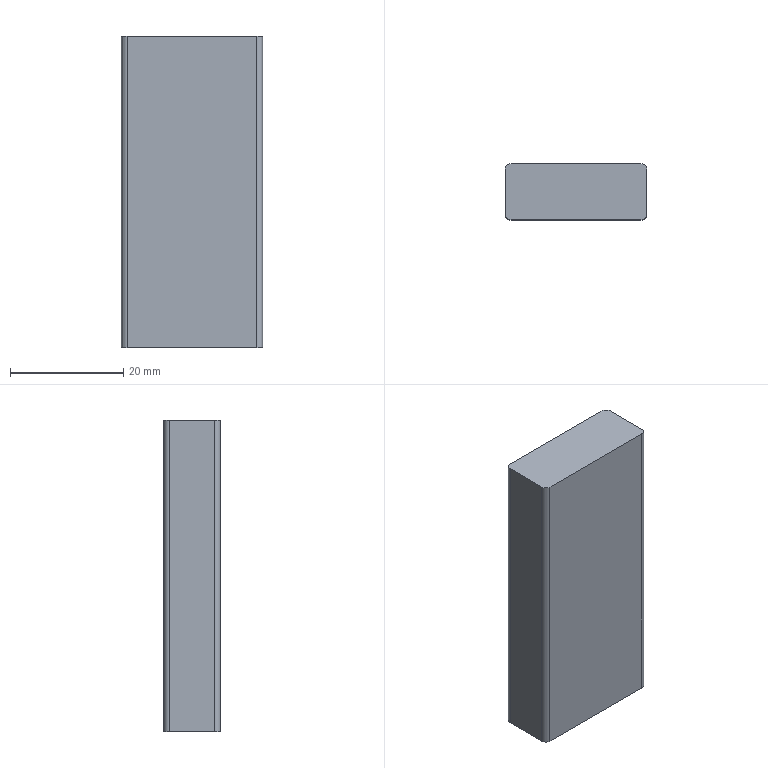Part | STEP file | 1 solid | 10 faces | box 24.97 x 9.97 x 55 mm | volume 13645 mm3 | plane 6 | cylinder 4 | commonest cylinder face diameters 2 x4
STEP:
#1=CARTESIAN_POINT('',(0.,0.,0.));
#2=DIRECTION('',(0.,0.,1.));
#3=DIRECTION('',(1.,0.,0.));
#4=AXIS2_PLACEMENT_3D('',#1,#2,#3);
#5=CARTESIAN_POINT('',(1277.232,396.43,43.619));
#6=VERTEX_POINT('',#5);
#7=CARTESIAN_POINT('',(1277.232,388.46,43.619));
#8=VERTEX_POINT('',#7);
#9=CARTESIAN_POINT('',(1277.232,397.445,43.619));
#10=DIRECTION('',(0.,-1.,0.));
#11=VECTOR('',#10,1.);
#12=LINE('',#9,#11);
#13=CARTESIAN_POINT('',(20683.4,-3580.314,43.619));
#14=DIRECTION('',(0.,0.,1.));
#15=DIRECTION('',(1.,0.,0.));
#16=AXIS2_PLACEMENT_3D('',#13,#14,#15);
#17=PLANE('',#16);
#18=CARTESIAN_POINT('',(-19406.168,3977.759));
#19=DIRECTION('',(0.,-1.));
#20=VECTOR('',#19,1.);
#21=LINE('',#18,#20);
#22=(GEOMETRIC_REPRESENTATION_CONTEXT(2)PARAMETRIC_REPRESENTATION_CONTEXT()REPRESENTATION_CONTEXT('',''));
#23=DEFINITIONAL_REPRESENTATION('',(#21),#22);
#24=PCURVE('',#17,#23);
#25=CARTESIAN_POINT('',(1277.232,397.445,426.319));
#26=DIRECTION('',(1.,0.,0.));
#27=DIRECTION('',(0.,0.,-1.));
#28=AXIS2_PLACEMENT_3D('',#25,#26,#27);
#29=PLANE('',#28);
#30=CARTESIAN_POINT('',(382.7,0.));
#31=DIRECTION('',(0.,-1.));
#32=VECTOR('',#31,1.);
#33=LINE('',#30,#32);
#34=(GEOMETRIC_REPRESENTATION_CONTEXT(2)PARAMETRIC_REPRESENTATION_CONTEXT()REPRESENTATION_CONTEXT('',''));
#35=DEFINITIONAL_REPRESENTATION('',(#33),#34);
#36=PCURVE('',#29,#35);
#37=SURFACE_CURVE('',#12,(#24,#36),.PCURVE_S1.);
#38=EDGE_CURVE('',#6,#8,#37,.T.);
#39=ORIENTED_EDGE('',*,*,#38,.F.);
#40=CARTESIAN_POINT('',(1276.232,397.43,43.619));
#41=VERTEX_POINT('',#40);
#42=CARTESIAN_POINT('',(1276.232,396.43,43.619));
#43=DIRECTION('',(0.,0.,1.));
#44=DIRECTION('',(-1.,0.,0.));
#45=AXIS2_PLACEMENT_3D('',#42,#43,#44);
#46=CIRCLE('',#45,1.);
#47=CARTESIAN_POINT('',(-19407.168,3976.744));
#48=DIRECTION('',(-1.,0.));
#49=AXIS2_PLACEMENT_2D('',#47,#48);
#50=CIRCLE('',#49,1.);
#51=(GEOMETRIC_REPRESENTATION_CONTEXT(2)PARAMETRIC_REPRESENTATION_CONTEXT()REPRESENTATION_CONTEXT('',''));
#52=DEFINITIONAL_REPRESENTATION('',(#50),#51);
#53=PCURVE('',#17,#52);
#54=CARTESIAN_POINT('',(1276.232,396.43,426.319));
#55=DIRECTION('',(0.,0.,-1.));
#56=DIRECTION('',(-1.,0.,0.));
#57=AXIS2_PLACEMENT_3D('',#54,#55,#56);
#58=CYLINDRICAL_SURFACE('',#57,1.);
#59=CARTESIAN_POINT('',(6.283,382.7));
#60=DIRECTION('',(-1.,0.));
#61=VECTOR('',#60,1.);
#62=LINE('',#59,#61);
#63=(GEOMETRIC_REPRESENTATION_CONTEXT(2)PARAMETRIC_REPRESENTATION_CONTEXT()REPRESENTATION_CONTEXT('',''));
#64=DEFINITIONAL_REPRESENTATION('',(#62),#63);
#65=PCURVE('',#58,#64);
#66=SURFACE_CURVE('',#46,(#53,#65),.PCURVE_S1.);
#67=EDGE_CURVE('',#6,#41,#66,.T.);
#68=ORIENTED_EDGE('',*,*,#67,.T.);
#69=CARTESIAN_POINT('',(1253.262,397.43,43.619));
#70=VERTEX_POINT('',#69);
#71=CARTESIAN_POINT('',(1252.247,397.43,43.619));
#72=DIRECTION('',(1.,0.,0.));
#73=VECTOR('',#72,1.);
#74=LINE('',#71,#73);
#75=CARTESIAN_POINT('',(-19431.153,3977.744));
#76=DIRECTION('',(1.,0.));
#77=VECTOR('',#76,1.);
#78=LINE('',#75,#77);
#79=(GEOMETRIC_REPRESENTATION_CONTEXT(2)PARAMETRIC_REPRESENTATION_CONTEXT()REPRESENTATION_CONTEXT('',''));
#80=DEFINITIONAL_REPRESENTATION('',(#78),#79);
#81=PCURVE('',#17,#80);
#82=CARTESIAN_POINT('',(1252.247,397.43,426.319));
#83=DIRECTION('',(0.,1.,0.));
#84=DIRECTION('',(0.,0.,-1.));
#85=AXIS2_PLACEMENT_3D('',#82,#83,#84);
#86=PLANE('',#85);
#87=CARTESIAN_POINT('',(382.7,0.));
#88=DIRECTION('',(0.,-1.));
#89=VECTOR('',#88,1.);
#90=LINE('',#87,#89);
#91=(GEOMETRIC_REPRESENTATION_CONTEXT(2)PARAMETRIC_REPRESENTATION_CONTEXT()REPRESENTATION_CONTEXT('',''));
#92=DEFINITIONAL_REPRESENTATION('',(#90),#91);
#93=PCURVE('',#86,#92);
#94=SURFACE_CURVE('',#74,(#81,#93),.PCURVE_S1.);
#95=EDGE_CURVE('',#70,#41,#94,.T.);
#96=ORIENTED_EDGE('',*,*,#95,.F.);
#97=CARTESIAN_POINT('',(1252.262,396.43,43.619));
#98=VERTEX_POINT('',#97);
#99=CARTESIAN_POINT('',(1253.262,396.43,43.619));
#100=DIRECTION('',(0.,0.,1.));
#101=DIRECTION('',(-1.,0.,0.));
#102=AXIS2_PLACEMENT_3D('',#99,#100,#101);
#103=CIRCLE('',#102,1.);
#104=CARTESIAN_POINT('',(-19430.138,3976.744));
#105=DIRECTION('',(-1.,0.));
#106=AXIS2_PLACEMENT_2D('',#104,#105);
#107=CIRCLE('',#106,1.);
#108=(GEOMETRIC_REPRESENTATION_CONTEXT(2)PARAMETRIC_REPRESENTATION_CONTEXT()REPRESENTATION_CONTEXT('',''));
#109=DEFINITIONAL_REPRESENTATION('',(#107),#108);
#110=PCURVE('',#17,#109);
#111=CARTESIAN_POINT('',(1253.262,396.43,426.319));
#112=DIRECTION('',(0.,0.,-1.));
#113=DIRECTION('',(-1.,0.,0.));
#114=AXIS2_PLACEMENT_3D('',#111,#112,#113);
#115=CYLINDRICAL_SURFACE('',#114,1.);
#116=CARTESIAN_POINT('',(6.283,382.7));
#117=DIRECTION('',(-1.,0.));
#118=VECTOR('',#117,1.);
#119=LINE('',#116,#118);
#120=(GEOMETRIC_REPRESENTATION_CONTEXT(2)PARAMETRIC_REPRESENTATION_CONTEXT()REPRESENTATION_CONTEXT('',''));
#121=DEFINITIONAL_REPRESENTATION('',(#119),#120);
#122=PCURVE('',#115,#121);
#123=SURFACE_CURVE('',#103,(#110,#122),.PCURVE_S1.);
#124=EDGE_CURVE('',#70,#98,#123,.T.);
#125=ORIENTED_EDGE('',*,*,#124,.T.);
#126=CARTESIAN_POINT('',(1252.262,388.46,43.619));
#127=VERTEX_POINT('',#126);
#128=CARTESIAN_POINT('',(1252.262,387.445,43.619));
#129=DIRECTION('',(0.,1.,0.));
#130=VECTOR('',#129,1.);
#131=LINE('',#128,#130);
#132=CARTESIAN_POINT('',(-19431.138,3967.759));
#133=DIRECTION('',(0.,1.));
#134=VECTOR('',#133,1.);
#135=LINE('',#132,#134);
#136=(GEOMETRIC_REPRESENTATION_CONTEXT(2)PARAMETRIC_REPRESENTATION_CONTEXT()REPRESENTATION_CONTEXT('',''));
#137=DEFINITIONAL_REPRESENTATION('',(#135),#136);
#138=PCURVE('',#17,#137);
#139=CARTESIAN_POINT('',(1252.262,387.445,426.319));
#140=DIRECTION('',(-1.,0.,0.));
#141=DIRECTION('',(0.,0.,1.));
#142=AXIS2_PLACEMENT_3D('',#139,#140,#141);
#143=PLANE('',#142);
#144=CARTESIAN_POINT('',(-382.7,0.));
#145=DIRECTION('',(0.,1.));
#146=VECTOR('',#145,1.);
#147=LINE('',#144,#146);
#148=(GEOMETRIC_REPRESENTATION_CONTEXT(2)PARAMETRIC_REPRESENTATION_CONTEXT()REPRESENTATION_CONTEXT('',''));
#149=DEFINITIONAL_REPRESENTATION('',(#147),#148);
#150=PCURVE('',#143,#149);
#151=SURFACE_CURVE('',#131,(#138,#150),.PCURVE_S1.);
#152=EDGE_CURVE('',#127,#98,#151,.T.);
#153=ORIENTED_EDGE('',*,*,#152,.F.);
#154=CARTESIAN_POINT('',(1253.262,387.46,43.619));
#155=VERTEX_POINT('',#154);
#156=CARTESIAN_POINT('',(1253.262,388.46,43.619));
#157=DIRECTION('',(0.,0.,1.));
#158=DIRECTION('',(-1.,0.,0.));
#159=AXIS2_PLACEMENT_3D('',#156,#157,#158);
#160=CIRCLE('',#159,1.);
#161=CARTESIAN_POINT('',(-19430.138,3968.774));
#162=DIRECTION('',(-1.,0.));
#163=AXIS2_PLACEMENT_2D('',#161,#162);
#164=CIRCLE('',#163,1.);
#165=(GEOMETRIC_REPRESENTATION_CONTEXT(2)PARAMETRIC_REPRESENTATION_CONTEXT()REPRESENTATION_CONTEXT('',''));
#166=DEFINITIONAL_REPRESENTATION('',(#164),#165);
#167=PCURVE('',#17,#166);
#168=CARTESIAN_POINT('',(1253.262,388.46,426.319));
#169=DIRECTION('',(0.,0.,-1.));
#170=DIRECTION('',(-1.,0.,0.));
#171=AXIS2_PLACEMENT_3D('',#168,#169,#170);
#172=CYLINDRICAL_SURFACE('',#171,1.);
#173=CARTESIAN_POINT('',(6.283,382.7));
#174=DIRECTION('',(-1.,0.));
#175=VECTOR('',#174,1.);
#176=LINE('',#173,#175);
#177=(GEOMETRIC_REPRESENTATION_CONTEXT(2)PARAMETRIC_REPRESENTATION_CONTEXT()REPRESENTATION_CONTEXT('',''));
#178=DEFINITIONAL_REPRESENTATION('',(#176),#177);
#179=PCURVE('',#172,#178);
#180=SURFACE_CURVE('',#160,(#167,#179),.PCURVE_S1.);
#181=EDGE_CURVE('',#127,#155,#180,.T.);
#182=ORIENTED_EDGE('',*,*,#181,.T.);
#183=CARTESIAN_POINT('',(1276.232,387.46,43.619));
#184=VERTEX_POINT('',#183);
#185=CARTESIAN_POINT('',(1277.247,387.46,43.619));
#186=DIRECTION('',(-1.,0.,0.));
#187=VECTOR('',#186,1.);
#188=LINE('',#185,#187);
#189=CARTESIAN_POINT('',(-19406.153,3967.774));
#190=DIRECTION('',(-1.,0.));
#191=VECTOR('',#190,1.);
#192=LINE('',#189,#191);
#193=(GEOMETRIC_REPRESENTATION_CONTEXT(2)PARAMETRIC_REPRESENTATION_CONTEXT()REPRESENTATION_CONTEXT('',''));
#194=DEFINITIONAL_REPRESENTATION('',(#192),#193);
#195=PCURVE('',#17,#194);
#196=CARTESIAN_POINT('',(1277.247,387.46,426.319));
#197=DIRECTION('',(0.,-1.,0.));
#198=DIRECTION('',(0.,0.,1.));
#199=AXIS2_PLACEMENT_3D('',#196,#197,#198);
#200=PLANE('',#199);
#201=CARTESIAN_POINT('',(-382.7,0.));
#202=DIRECTION('',(0.,1.));
#203=VECTOR('',#202,1.);
#204=LINE('',#201,#203);
#205=(GEOMETRIC_REPRESENTATION_CONTEXT(2)PARAMETRIC_REPRESENTATION_CONTEXT()REPRESENTATION_CONTEXT('',''));
#206=DEFINITIONAL_REPRESENTATION('',(#204),#205);
#207=PCURVE('',#200,#206);
#208=SURFACE_CURVE('',#188,(#195,#207),.PCURVE_S1.);
#209=EDGE_CURVE('',#184,#155,#208,.T.);
#210=ORIENTED_EDGE('',*,*,#209,.F.);
#211=CARTESIAN_POINT('',(1276.232,388.46,43.619));
#212=DIRECTION('',(0.,0.,1.));
#213=DIRECTION('',(-1.,0.,0.));
#214=AXIS2_PLACEMENT_3D('',#211,#212,#213);
#215=CIRCLE('',#214,1.);
#216=CARTESIAN_POINT('',(-19407.168,3968.774));
#217=DIRECTION('',(-1.,0.));
#218=AXIS2_PLACEMENT_2D('',#216,#217);
#219=CIRCLE('',#218,1.);
#220=(GEOMETRIC_REPRESENTATION_CONTEXT(2)PARAMETRIC_REPRESENTATION_CONTEXT()REPRESENTATION_CONTEXT('',''));
#221=DEFINITIONAL_REPRESENTATION('',(#219),#220);
#222=PCURVE('',#17,#221);
#223=CARTESIAN_POINT('',(1276.232,388.46,426.319));
#224=DIRECTION('',(0.,0.,-1.));
#225=DIRECTION('',(-1.,0.,0.));
#226=AXIS2_PLACEMENT_3D('',#223,#224,#225);
#227=CYLINDRICAL_SURFACE('',#226,1.);
#228=CARTESIAN_POINT('',(6.283,382.7));
#229=DIRECTION('',(-1.,0.));
#230=VECTOR('',#229,1.);
#231=LINE('',#228,#230);
#232=(GEOMETRIC_REPRESENTATION_CONTEXT(2)PARAMETRIC_REPRESENTATION_CONTEXT()REPRESENTATION_CONTEXT('',''));
#233=DEFINITIONAL_REPRESENTATION('',(#231),#232);
#234=PCURVE('',#227,#233);
#235=SURFACE_CURVE('',#215,(#222,#234),.PCURVE_S1.);
#236=EDGE_CURVE('',#184,#8,#235,.T.);
#237=ORIENTED_EDGE('',*,*,#236,.T.);
#238=EDGE_LOOP('',(#39,#68,#96,#125,#153,#182,#210,#237));
#239=FACE_BOUND('',#238,.T.);
#240=ADVANCED_FACE('',(#239),#17,.T.);
#241=ORIENTED_EDGE('',*,*,#152,.T.);
#242=CARTESIAN_POINT('',(1252.262,396.43,-11.381));
#243=VERTEX_POINT('',#242);
#244=CARTESIAN_POINT('',(1252.262,396.43,426.319));
#245=DIRECTION('',(0.,0.,-1.));
#246=VECTOR('',#245,1.);
#247=LINE('',#244,#246);
#248=CARTESIAN_POINT('',(0.,8.985));
#249=DIRECTION('',(-1.,0.));
#250=VECTOR('',#249,1.);
#251=LINE('',#248,#250);
#252=(GEOMETRIC_REPRESENTATION_CONTEXT(2)PARAMETRIC_REPRESENTATION_CONTEXT()REPRESENTATION_CONTEXT('',''));
#253=DEFINITIONAL_REPRESENTATION('',(#251),#252);
#254=PCURVE('',#143,#253);
#255=CARTESIAN_POINT('',(0.,0.));
#256=DIRECTION('',(0.,1.));
#257=VECTOR('',#256,1.);
#258=LINE('',#255,#257);
#259=(GEOMETRIC_REPRESENTATION_CONTEXT(2)PARAMETRIC_REPRESENTATION_CONTEXT()REPRESENTATION_CONTEXT('',''));
#260=DEFINITIONAL_REPRESENTATION('',(#258),#259);
#261=PCURVE('',#115,#260);
#262=SURFACE_CURVE('',#247,(#254,#261),.PCURVE_S1.);
#263=EDGE_CURVE('',#98,#243,#262,.T.);
#264=ORIENTED_EDGE('',*,*,#263,.T.);
#265=CARTESIAN_POINT('',(1252.262,388.46,-11.381));
#266=VERTEX_POINT('',#265);
#267=CARTESIAN_POINT('',(1252.262,-3580.314,-11.381));
#268=DIRECTION('',(0.,1.,0.));
#269=VECTOR('',#268,1.);
#270=LINE('',#267,#269);
#271=CARTESIAN_POINT('',(-437.7,-3967.759));
#272=DIRECTION('',(0.,1.));
#273=VECTOR('',#272,1.);
#274=LINE('',#271,#273);
#275=(GEOMETRIC_REPRESENTATION_CONTEXT(2)PARAMETRIC_REPRESENTATION_CONTEXT()REPRESENTATION_CONTEXT('',''));
#276=DEFINITIONAL_REPRESENTATION('',(#274),#275);
#277=PCURVE('',#143,#276);
#278=CARTESIAN_POINT('',(18446.131,-3580.314,-11.381));
#279=DIRECTION('',(0.,0.,-1.));
#280=DIRECTION('',(-1.,0.,0.));
#281=AXIS2_PLACEMENT_3D('',#278,#279,#280);
#282=PLANE('',#281);
#283=CARTESIAN_POINT('',(17193.869,0.));
#284=DIRECTION('',(0.,1.));
#285=VECTOR('',#284,1.);
#286=LINE('',#283,#285);
#287=(GEOMETRIC_REPRESENTATION_CONTEXT(2)PARAMETRIC_REPRESENTATION_CONTEXT()REPRESENTATION_CONTEXT('',''));
#288=DEFINITIONAL_REPRESENTATION('',(#286),#287);
#289=PCURVE('',#282,#288);
#290=SURFACE_CURVE('',#270,(#277,#289),.PCURVE_S1.);
#291=EDGE_CURVE('',#266,#243,#290,.T.);
#292=ORIENTED_EDGE('',*,*,#291,.F.);
#293=CARTESIAN_POINT('',(1252.262,388.46,426.319));
#294=DIRECTION('',(0.,0.,1.));
#295=VECTOR('',#294,1.);
#296=LINE('',#293,#295);
#297=CARTESIAN_POINT('',(0.,1.015));
#298=DIRECTION('',(1.,0.));
#299=VECTOR('',#298,1.);
#300=LINE('',#297,#299);
#301=(GEOMETRIC_REPRESENTATION_CONTEXT(2)PARAMETRIC_REPRESENTATION_CONTEXT()REPRESENTATION_CONTEXT('',''));
#302=DEFINITIONAL_REPRESENTATION('',(#300),#301);
#303=PCURVE('',#143,#302);
#304=CARTESIAN_POINT('',(6.283,0.));
#305=DIRECTION('',(0.,-1.));
#306=VECTOR('',#305,1.);
#307=LINE('',#304,#306);
#308=(GEOMETRIC_REPRESENTATION_CONTEXT(2)PARAMETRIC_REPRESENTATION_CONTEXT()REPRESENTATION_CONTEXT('',''));
#309=DEFINITIONAL_REPRESENTATION('',(#307),#308);
#310=PCURVE('',#172,#309);
#311=SURFACE_CURVE('',#296,(#303,#310),.PCURVE_S1.);
#312=EDGE_CURVE('',#266,#127,#311,.T.);
#313=ORIENTED_EDGE('',*,*,#312,.T.);
#314=EDGE_LOOP('',(#241,#264,#292,#313));
#315=FACE_BOUND('',#314,.T.);
#316=ADVANCED_FACE('',(#315),#143,.T.);
#317=CARTESIAN_POINT('',(1253.262,397.43,-11.381));
#318=VERTEX_POINT('',#317);
#319=CARTESIAN_POINT('',(1276.232,397.43,-11.381));
#320=VERTEX_POINT('',#319);
#321=CARTESIAN_POINT('',(18446.131,397.43,-11.381));
#322=DIRECTION('',(1.,0.,0.));
#323=VECTOR('',#322,1.);
#324=LINE('',#321,#323);
#325=CARTESIAN_POINT('',(0.,3977.744));
#326=DIRECTION('',(-1.,0.));
#327=VECTOR('',#326,1.);
#328=LINE('',#325,#327);
#329=(GEOMETRIC_REPRESENTATION_CONTEXT(2)PARAMETRIC_REPRESENTATION_CONTEXT()REPRESENTATION_CONTEXT('',''));
#330=DEFINITIONAL_REPRESENTATION('',(#328),#329);
#331=PCURVE('',#282,#330);
#332=CARTESIAN_POINT('',(437.7,-17193.884));
#333=DIRECTION('',(0.,-1.));
#334=VECTOR('',#333,1.);
#335=LINE('',#332,#334);
#336=(GEOMETRIC_REPRESENTATION_CONTEXT(2)PARAMETRIC_REPRESENTATION_CONTEXT()REPRESENTATION_CONTEXT('',''));
#337=DEFINITIONAL_REPRESENTATION('',(#335),#336);
#338=PCURVE('',#86,#337);
#339=SURFACE_CURVE('',#324,(#331,#338),.PCURVE_S1.);
#340=EDGE_CURVE('',#318,#320,#339,.T.);
#341=ORIENTED_EDGE('',*,*,#340,.T.);
#342=CARTESIAN_POINT('',(1277.232,396.43,-11.381));
#343=VERTEX_POINT('',#342);
#344=CARTESIAN_POINT('',(1276.232,396.43,-11.381));
#345=DIRECTION('',(0.,0.,-1.));
#346=DIRECTION('',(-1.,0.,0.));
#347=AXIS2_PLACEMENT_3D('',#344,#345,#346);
#348=CIRCLE('',#347,1.);
#349=CARTESIAN_POINT('',(17169.899,3976.744));
#350=DIRECTION('',(1.,0.));
#351=AXIS2_PLACEMENT_2D('',#349,#350);
#352=CIRCLE('',#351,1.);
#353=(GEOMETRIC_REPRESENTATION_CONTEXT(2)PARAMETRIC_REPRESENTATION_CONTEXT()REPRESENTATION_CONTEXT('',''));
#354=DEFINITIONAL_REPRESENTATION('',(#352),#353);
#355=PCURVE('',#282,#354);
#356=CARTESIAN_POINT('',(0.,437.7));
#357=DIRECTION('',(1.,0.));
#358=VECTOR('',#357,1.);
#359=LINE('',#356,#358);
#360=(GEOMETRIC_REPRESENTATION_CONTEXT(2)PARAMETRIC_REPRESENTATION_CONTEXT()REPRESENTATION_CONTEXT('',''));
#361=DEFINITIONAL_REPRESENTATION('',(#359),#360);
#362=PCURVE('',#58,#361);
#363=SURFACE_CURVE('',#348,(#355,#362),.PCURVE_S1.);
#364=EDGE_CURVE('',#320,#343,#363,.T.);
#365=ORIENTED_EDGE('',*,*,#364,.T.);
#366=CARTESIAN_POINT('',(1277.232,388.46,-11.381));
#367=VERTEX_POINT('',#366);
#368=CARTESIAN_POINT('',(1277.232,-3580.314,-11.381));
#369=DIRECTION('',(0.,-1.,0.));
#370=VECTOR('',#369,1.);
#371=LINE('',#368,#370);
#372=CARTESIAN_POINT('',(17168.899,0.));
#373=DIRECTION('',(0.,-1.));
#374=VECTOR('',#373,1.);
#375=LINE('',#372,#374);
#376=(GEOMETRIC_REPRESENTATION_CONTEXT(2)PARAMETRIC_REPRESENTATION_CONTEXT()REPRESENTATION_CONTEXT('',''));
#377=DEFINITIONAL_REPRESENTATION('',(#375),#376);
#378=PCURVE('',#282,#377);
#379=CARTESIAN_POINT('',(437.7,-3977.759));
#380=DIRECTION('',(0.,-1.));
#381=VECTOR('',#380,1.);
#382=LINE('',#379,#381);
#383=(GEOMETRIC_REPRESENTATION_CONTEXT(2)PARAMETRIC_REPRESENTATION_CONTEXT()REPRESENTATION_CONTEXT('',''));
#384=DEFINITIONAL_REPRESENTATION('',(#382),#383);
#385=PCURVE('',#29,#384);
#386=SURFACE_CURVE('',#371,(#378,#385),.PCURVE_S1.);
#387=EDGE_CURVE('',#343,#367,#386,.T.);
#388=ORIENTED_EDGE('',*,*,#387,.T.);
#389=CARTESIAN_POINT('',(1276.232,387.46,-11.381));
#390=VERTEX_POINT('',#389);
#391=CARTESIAN_POINT('',(1276.232,388.46,-11.381));
#392=DIRECTION('',(0.,0.,-1.));
#393=DIRECTION('',(-1.,0.,0.));
#394=AXIS2_PLACEMENT_3D('',#391,#392,#393);
#395=CIRCLE('',#394,1.);
#396=CARTESIAN_POINT('',(17169.899,3968.774));
#397=DIRECTION('',(1.,0.));
#398=AXIS2_PLACEMENT_2D('',#396,#397);
#399=CIRCLE('',#398,1.);
#400=(GEOMETRIC_REPRESENTATION_CONTEXT(2)PARAMETRIC_REPRESENTATION_CONTEXT()REPRESENTATION_CONTEXT('',''));
#401=DEFINITIONAL_REPRESENTATION('',(#399),#400);
#402=PCURVE('',#282,#401);
#403=CARTESIAN_POINT('',(0.,437.7));
#404=DIRECTION('',(1.,0.));
#405=VECTOR('',#404,1.);
#406=LINE('',#403,#405);
#407=(GEOMETRIC_REPRESENTATION_CONTEXT(2)PARAMETRIC_REPRESENTATION_CONTEXT()REPRESENTATION_CONTEXT('',''));
#408=DEFINITIONAL_REPRESENTATION('',(#406),#407);
#409=PCURVE('',#227,#408);
#410=SURFACE_CURVE('',#395,(#402,#409),.PCURVE_S1.);
#411=EDGE_CURVE('',#367,#390,#410,.T.);
#412=ORIENTED_EDGE('',*,*,#411,.T.);
#413=CARTESIAN_POINT('',(1253.262,387.46,-11.381));
#414=VERTEX_POINT('',#413);
#415=CARTESIAN_POINT('',(18446.131,387.46,-11.381));
#416=DIRECTION('',(-1.,0.,0.));
#417=VECTOR('',#416,1.);
#418=LINE('',#415,#417);
#419=CARTESIAN_POINT('',(0.,3967.774));
#420=DIRECTION('',(1.,0.));
#421=VECTOR('',#420,1.);
#422=LINE('',#419,#421);
#423=(GEOMETRIC_REPRESENTATION_CONTEXT(2)PARAMETRIC_REPRESENTATION_CONTEXT()REPRESENTATION_CONTEXT('',''));
#424=DEFINITIONAL_REPRESENTATION('',(#422),#423);
#425=PCURVE('',#282,#424);
#426=CARTESIAN_POINT('',(-437.7,-17168.884));
#427=DIRECTION('',(0.,1.));
#428=VECTOR('',#427,1.);
#429=LINE('',#426,#428);
#430=(GEOMETRIC_REPRESENTATION_CONTEXT(2)PARAMETRIC_REPRESENTATION_CONTEXT()REPRESENTATION_CONTEXT('',''));
#431=DEFINITIONAL_REPRESENTATION('',(#429),#430);
#432=PCURVE('',#200,#431);
#433=SURFACE_CURVE('',#418,(#425,#432),.PCURVE_S1.);
#434=EDGE_CURVE('',#390,#414,#433,.T.);
#435=ORIENTED_EDGE('',*,*,#434,.T.);
#436=CARTESIAN_POINT('',(1253.262,388.46,-11.381));
#437=DIRECTION('',(0.,0.,-1.));
#438=DIRECTION('',(-1.,0.,0.));
#439=AXIS2_PLACEMENT_3D('',#436,#437,#438);
#440=CIRCLE('',#439,1.);
#441=CARTESIAN_POINT('',(17192.869,3968.774));
#442=DIRECTION('',(1.,0.));
#443=AXIS2_PLACEMENT_2D('',#441,#442);
#444=CIRCLE('',#443,1.);
#445=(GEOMETRIC_REPRESENTATION_CONTEXT(2)PARAMETRIC_REPRESENTATION_CONTEXT()REPRESENTATION_CONTEXT('',''));
#446=DEFINITIONAL_REPRESENTATION('',(#444),#445);
#447=PCURVE('',#282,#446);
#448=CARTESIAN_POINT('',(0.,437.7));
#449=DIRECTION('',(1.,0.));
#450=VECTOR('',#449,1.);
#451=LINE('',#448,#450);
#452=(GEOMETRIC_REPRESENTATION_CONTEXT(2)PARAMETRIC_REPRESENTATION_CONTEXT()REPRESENTATION_CONTEXT('',''));
#453=DEFINITIONAL_REPRESENTATION('',(#451),#452);
#454=PCURVE('',#172,#453);
#455=SURFACE_CURVE('',#440,(#447,#454),.PCURVE_S1.);
#456=EDGE_CURVE('',#414,#266,#455,.T.);
#457=ORIENTED_EDGE('',*,*,#456,.T.);
#458=ORIENTED_EDGE('',*,*,#291,.T.);
#459=CARTESIAN_POINT('',(1253.262,396.43,-11.381));
#460=DIRECTION('',(0.,0.,-1.));
#461=DIRECTION('',(-1.,0.,0.));
#462=AXIS2_PLACEMENT_3D('',#459,#460,#461);
#463=CIRCLE('',#462,1.);
#464=CARTESIAN_POINT('',(17192.869,3976.744));
#465=DIRECTION('',(1.,0.));
#466=AXIS2_PLACEMENT_2D('',#464,#465);
#467=CIRCLE('',#466,1.);
#468=(GEOMETRIC_REPRESENTATION_CONTEXT(2)PARAMETRIC_REPRESENTATION_CONTEXT()REPRESENTATION_CONTEXT('',''));
#469=DEFINITIONAL_REPRESENTATION('',(#467),#468);
#470=PCURVE('',#282,#469);
#471=CARTESIAN_POINT('',(0.,437.7));
#472=DIRECTION('',(1.,0.));
#473=VECTOR('',#472,1.);
#474=LINE('',#471,#473);
#475=(GEOMETRIC_REPRESENTATION_CONTEXT(2)PARAMETRIC_REPRESENTATION_CONTEXT()REPRESENTATION_CONTEXT('',''));
#476=DEFINITIONAL_REPRESENTATION('',(#474),#475);
#477=PCURVE('',#115,#476);
#478=SURFACE_CURVE('',#463,(#470,#477),.PCURVE_S1.);
#479=EDGE_CURVE('',#243,#318,#478,.T.);
#480=ORIENTED_EDGE('',*,*,#479,.T.);
#481=EDGE_LOOP('',(#341,#365,#388,#412,#435,#457,#458,#480));
#482=FACE_BOUND('',#481,.T.);
#483=ADVANCED_FACE('',(#482),#282,.T.);
#484=ORIENTED_EDGE('',*,*,#209,.T.);
#485=CARTESIAN_POINT('',(1253.262,387.46,426.319));
#486=DIRECTION('',(0.,0.,-1.));
#487=VECTOR('',#486,1.);
#488=LINE('',#485,#487);
#489=CARTESIAN_POINT('',(0.,23.985));
#490=DIRECTION('',(-1.,0.));
#491=VECTOR('',#490,1.);
#492=LINE('',#489,#491);
#493=(GEOMETRIC_REPRESENTATION_CONTEXT(2)PARAMETRIC_REPRESENTATION_CONTEXT()REPRESENTATION_CONTEXT('',''));
#494=DEFINITIONAL_REPRESENTATION('',(#492),#493);
#495=PCURVE('',#200,#494);
#496=CARTESIAN_POINT('',(4.712,0.));
#497=DIRECTION('',(0.,1.));
#498=VECTOR('',#497,1.);
#499=LINE('',#496,#498);
#500=(GEOMETRIC_REPRESENTATION_CONTEXT(2)PARAMETRIC_REPRESENTATION_CONTEXT()REPRESENTATION_CONTEXT('',''));
#501=DEFINITIONAL_REPRESENTATION('',(#499),#500);
#502=PCURVE('',#172,#501);
#503=SURFACE_CURVE('',#488,(#495,#502),.PCURVE_S1.);
#504=EDGE_CURVE('',#155,#414,#503,.T.);
#505=ORIENTED_EDGE('',*,*,#504,.T.);
#506=ORIENTED_EDGE('',*,*,#434,.F.);
#507=CARTESIAN_POINT('',(1276.232,387.46,426.319));
#508=DIRECTION('',(0.,0.,1.));
#509=VECTOR('',#508,1.);
#510=LINE('',#507,#509);
#511=CARTESIAN_POINT('',(0.,1.015));
#512=DIRECTION('',(1.,0.));
#513=VECTOR('',#512,1.);
#514=LINE('',#511,#513);
#515=(GEOMETRIC_REPRESENTATION_CONTEXT(2)PARAMETRIC_REPRESENTATION_CONTEXT()REPRESENTATION_CONTEXT('',''));
#516=DEFINITIONAL_REPRESENTATION('',(#514),#515);
#517=PCURVE('',#200,#516);
#518=CARTESIAN_POINT('',(4.712,0.));
#519=DIRECTION('',(0.,-1.));
#520=VECTOR('',#519,1.);
#521=LINE('',#518,#520);
#522=(GEOMETRIC_REPRESENTATION_CONTEXT(2)PARAMETRIC_REPRESENTATION_CONTEXT()REPRESENTATION_CONTEXT('',''));
#523=DEFINITIONAL_REPRESENTATION('',(#521),#522);
#524=PCURVE('',#227,#523);
#525=SURFACE_CURVE('',#510,(#517,#524),.PCURVE_S1.);
#526=EDGE_CURVE('',#390,#184,#525,.T.);
#527=ORIENTED_EDGE('',*,*,#526,.T.);
#528=EDGE_LOOP('',(#484,#505,#506,#527));
#529=FACE_BOUND('',#528,.T.);
#530=ADVANCED_FACE('',(#529),#200,.T.);
#531=ORIENTED_EDGE('',*,*,#95,.T.);
#532=CARTESIAN_POINT('',(1276.232,397.43,426.319));
#533=DIRECTION('',(0.,0.,-1.));
#534=VECTOR('',#533,1.);
#535=LINE('',#532,#534);
#536=CARTESIAN_POINT('',(0.,-23.985));
#537=DIRECTION('',(1.,0.));
#538=VECTOR('',#537,1.);
#539=LINE('',#536,#538);
#540=(GEOMETRIC_REPRESENTATION_CONTEXT(2)PARAMETRIC_REPRESENTATION_CONTEXT()REPRESENTATION_CONTEXT('',''));
#541=DEFINITIONAL_REPRESENTATION('',(#539),#540);
#542=PCURVE('',#86,#541);
#543=CARTESIAN_POINT('',(1.571,0.));
#544=DIRECTION('',(0.,1.));
#545=VECTOR('',#544,1.);
#546=LINE('',#543,#545);
#547=(GEOMETRIC_REPRESENTATION_CONTEXT(2)PARAMETRIC_REPRESENTATION_CONTEXT()REPRESENTATION_CONTEXT('',''));
#548=DEFINITIONAL_REPRESENTATION('',(#546),#547);
#549=PCURVE('',#58,#548);
#550=SURFACE_CURVE('',#535,(#542,#549),.PCURVE_S1.);
#551=EDGE_CURVE('',#41,#320,#550,.T.);
#552=ORIENTED_EDGE('',*,*,#551,.T.);
#553=ORIENTED_EDGE('',*,*,#340,.F.);
#554=CARTESIAN_POINT('',(1253.262,397.43,426.319));
#555=DIRECTION('',(0.,0.,1.));
#556=VECTOR('',#555,1.);
#557=LINE('',#554,#556);
#558=CARTESIAN_POINT('',(0.,-1.015));
#559=DIRECTION('',(-1.,0.));
#560=VECTOR('',#559,1.);
#561=LINE('',#558,#560);
#562=(GEOMETRIC_REPRESENTATION_CONTEXT(2)PARAMETRIC_REPRESENTATION_CONTEXT()REPRESENTATION_CONTEXT('',''));
#563=DEFINITIONAL_REPRESENTATION('',(#561),#562);
#564=PCURVE('',#86,#563);
#565=CARTESIAN_POINT('',(1.571,0.));
#566=DIRECTION('',(0.,-1.));
#567=VECTOR('',#566,1.);
#568=LINE('',#565,#567);
#569=(GEOMETRIC_REPRESENTATION_CONTEXT(2)PARAMETRIC_REPRESENTATION_CONTEXT()REPRESENTATION_CONTEXT('',''));
#570=DEFINITIONAL_REPRESENTATION('',(#568),#569);
#571=PCURVE('',#115,#570);
#572=SURFACE_CURVE('',#557,(#564,#571),.PCURVE_S1.);
#573=EDGE_CURVE('',#318,#70,#572,.T.);
#574=ORIENTED_EDGE('',*,*,#573,.T.);
#575=EDGE_LOOP('',(#531,#552,#553,#574));
#576=FACE_BOUND('',#575,.T.);
#577=ADVANCED_FACE('',(#576),#86,.T.);
#578=ORIENTED_EDGE('',*,*,#387,.F.);
#579=CARTESIAN_POINT('',(1277.232,396.43,426.319));
#580=DIRECTION('',(0.,0.,1.));
#581=VECTOR('',#580,1.);
#582=LINE('',#579,#581);
#583=CARTESIAN_POINT('',(0.,-1.015));
#584=DIRECTION('',(-1.,0.));
#585=VECTOR('',#584,1.);
#586=LINE('',#583,#585);
#587=(GEOMETRIC_REPRESENTATION_CONTEXT(2)PARAMETRIC_REPRESENTATION_CONTEXT()REPRESENTATION_CONTEXT('',''));
#588=DEFINITIONAL_REPRESENTATION('',(#586),#587);
#589=PCURVE('',#29,#588);
#590=CARTESIAN_POINT('',(3.142,0.));
#591=DIRECTION('',(0.,-1.));
#592=VECTOR('',#591,1.);
#593=LINE('',#590,#592);
#594=(GEOMETRIC_REPRESENTATION_CONTEXT(2)PARAMETRIC_REPRESENTATION_CONTEXT()REPRESENTATION_CONTEXT('',''));
#595=DEFINITIONAL_REPRESENTATION('',(#593),#594);
#596=PCURVE('',#58,#595);
#597=SURFACE_CURVE('',#582,(#589,#596),.PCURVE_S1.);
#598=EDGE_CURVE('',#343,#6,#597,.T.);
#599=ORIENTED_EDGE('',*,*,#598,.T.);
#600=ORIENTED_EDGE('',*,*,#38,.T.);
#601=CARTESIAN_POINT('',(1277.232,388.46,426.319));
#602=DIRECTION('',(0.,0.,-1.));
#603=VECTOR('',#602,1.);
#604=LINE('',#601,#603);
#605=CARTESIAN_POINT('',(0.,-8.985));
#606=DIRECTION('',(1.,0.));
#607=VECTOR('',#606,1.);
#608=LINE('',#605,#607);
#609=(GEOMETRIC_REPRESENTATION_CONTEXT(2)PARAMETRIC_REPRESENTATION_CONTEXT()REPRESENTATION_CONTEXT('',''));
#610=DEFINITIONAL_REPRESENTATION('',(#608),#609);
#611=PCURVE('',#29,#610);
#612=CARTESIAN_POINT('',(3.142,0.));
#613=DIRECTION('',(0.,1.));
#614=VECTOR('',#613,1.);
#615=LINE('',#612,#614);
#616=(GEOMETRIC_REPRESENTATION_CONTEXT(2)PARAMETRIC_REPRESENTATION_CONTEXT()REPRESENTATION_CONTEXT('',''));
#617=DEFINITIONAL_REPRESENTATION('',(#615),#616);
#618=PCURVE('',#227,#617);
#619=SURFACE_CURVE('',#604,(#611,#618),.PCURVE_S1.);
#620=EDGE_CURVE('',#8,#367,#619,.T.);
#621=ORIENTED_EDGE('',*,*,#620,.T.);
#622=EDGE_LOOP('',(#578,#599,#600,#621));
#623=FACE_BOUND('',#622,.T.);
#624=ADVANCED_FACE('',(#623),#29,.T.);
#625=ORIENTED_EDGE('',*,*,#67,.F.);
#626=ORIENTED_EDGE('',*,*,#598,.F.);
#627=ORIENTED_EDGE('',*,*,#364,.F.);
#628=ORIENTED_EDGE('',*,*,#551,.F.);
#629=EDGE_LOOP('',(#625,#626,#627,#628));
#630=FACE_BOUND('',#629,.T.);
#631=ADVANCED_FACE('',(#630),#58,.T.);
#632=ORIENTED_EDGE('',*,*,#124,.F.);
#633=ORIENTED_EDGE('',*,*,#573,.F.);
#634=ORIENTED_EDGE('',*,*,#479,.F.);
#635=ORIENTED_EDGE('',*,*,#263,.F.);
#636=EDGE_LOOP('',(#632,#633,#634,#635));
#637=FACE_BOUND('',#636,.T.);
#638=ADVANCED_FACE('',(#637),#115,.T.);
#639=ORIENTED_EDGE('',*,*,#181,.F.);
#640=ORIENTED_EDGE('',*,*,#312,.F.);
#641=ORIENTED_EDGE('',*,*,#456,.F.);
#642=ORIENTED_EDGE('',*,*,#504,.F.);
#643=EDGE_LOOP('',(#639,#640,#641,#642));
#644=FACE_BOUND('',#643,.T.);
#645=ADVANCED_FACE('',(#644),#172,.T.);
#646=ORIENTED_EDGE('',*,*,#236,.F.);
#647=ORIENTED_EDGE('',*,*,#526,.F.);
#648=ORIENTED_EDGE('',*,*,#411,.F.);
#649=ORIENTED_EDGE('',*,*,#620,.F.);
#650=EDGE_LOOP('',(#646,#647,#648,#649));
#651=FACE_BOUND('',#650,.T.);
#652=ADVANCED_FACE('',(#651),#227,.T.);
#653=CLOSED_SHELL('',(#240,#316,#483,#530,#577,#624,#631,#638,#645,#652));
#654=MANIFOLD_SOLID_BREP('',#653);
#655=(LENGTH_UNIT()NAMED_UNIT(*)SI_UNIT(.MILLI.,.METRE.));
#656=UNCERTAINTY_MEASURE_WITH_UNIT(LENGTH_MEASURE(0.0000001),#655,'','');
#657=(NAMED_UNIT(*)PLANE_ANGLE_UNIT()SI_UNIT($,.RADIAN.));
#658=(NAMED_UNIT(*)SI_UNIT($,.STERADIAN.)SOLID_ANGLE_UNIT());
#659=(GEOMETRIC_REPRESENTATION_CONTEXT(3)GLOBAL_UNCERTAINTY_ASSIGNED_CONTEXT((#656))GLOBAL_UNIT_ASSIGNED_CONTEXT((#655,#657,#658))REPRESENTATION_CONTEXT('',''));
#660=ADVANCED_BREP_SHAPE_REPRESENTATION('',(#4,#654),#659);